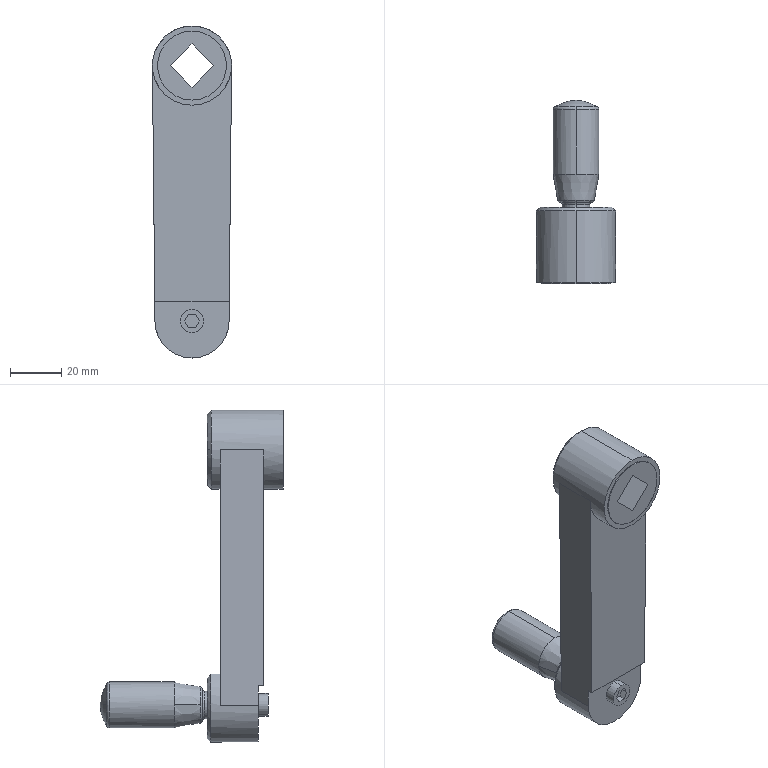Part | SolidWorks | features BaseBody 1 | 1 solid | 83 faces | box 31 x 72 x 130 mm | volume 55783 mm3 | plane 38 | cylinder 27 | spline 10 | cone 6 | torus 2 | commonest cylinder face diameters 3 x3 23 x3 2 x2 5.2 x2 9 x2 10.8 x2